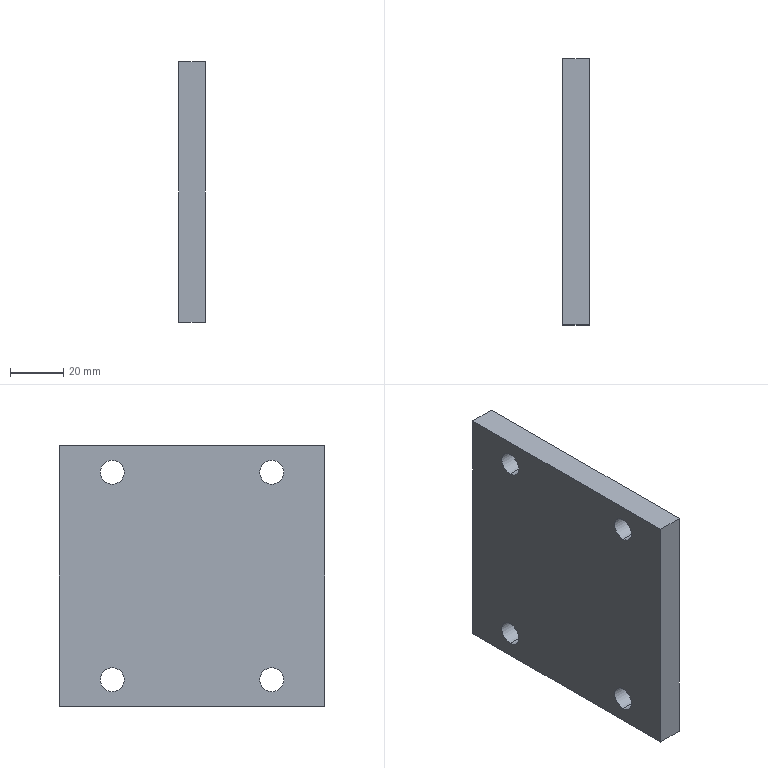Part | SolidWorks | features Extrusion 1, HoleWzd 1 | 1 solid | 14 faces | box 10 x 100 x 98 mm | volume 95455 mm3 | cylinder 8 | plane 6 | commonest cylinder face diameters 9 x8
STEP:
#1=CARTESIAN_POINT('',(0.,30.,43.5));
#2=VERTEX_POINT('',#1);
#3=CARTESIAN_POINT('',(0.,30.,34.5));
#4=VERTEX_POINT('',#3);
#5=CARTESIAN_POINT('',(0.,30.,39.));
#6=DIRECTION('',(1.,0.,0.));
#7=DIRECTION('',(0.,0.,-1.));
#8=AXIS2_PLACEMENT_3D('',#5,#6,#7);
#9=CIRCLE('',#8,4.5);
#10=EDGE_CURVE('',#2,#4,#9,.T.);
#11=ORIENTED_EDGE('',*,*,#10,.F.);
#12=CARTESIAN_POINT('',(10.,30.,43.5));
#13=VERTEX_POINT('',#12);
#14=CARTESIAN_POINT('',(10.,30.,43.5));
#15=DIRECTION('',(1.,0.,0.));
#16=VECTOR('',#15,1000.);
#17=LINE('',#14,#16);
#18=EDGE_CURVE('',#2,#13,#17,.T.);
#19=ORIENTED_EDGE('',*,*,#18,.T.);
#20=CARTESIAN_POINT('',(10.,30.,34.5));
#21=VERTEX_POINT('',#20);
#22=CARTESIAN_POINT('',(10.,30.,39.));
#23=DIRECTION('',(1.,0.,0.));
#24=DIRECTION('',(0.,0.,-1.));
#25=AXIS2_PLACEMENT_3D('',#22,#23,#24);
#26=CIRCLE('',#25,4.5);
#27=EDGE_CURVE('',#13,#21,#26,.T.);
#28=ORIENTED_EDGE('',*,*,#27,.T.);
#29=CARTESIAN_POINT('',(10.,30.,34.5));
#30=DIRECTION('',(1.,0.,0.));
#31=VECTOR('',#30,1000.);
#32=LINE('',#29,#31);
#33=EDGE_CURVE('',#4,#21,#32,.T.);
#34=ORIENTED_EDGE('',*,*,#33,.F.);
#35=EDGE_LOOP('',(#11,#19,#28,#34));
#36=FACE_OUTER_BOUND('',#35,.T.);
#37=CARTESIAN_POINT('',(10.,30.,39.));
#38=DIRECTION('',(1.,0.,0.));
#39=DIRECTION('',(0.,0.,-1.));
#40=AXIS2_PLACEMENT_3D('',#37,#38,#39);
#41=CYLINDRICAL_SURFACE('',#40,4.5);
#42=ADVANCED_FACE('',(#36),#41,.F.);
#43=CARTESIAN_POINT('',(0.,30.,-34.5));
#44=VERTEX_POINT('',#43);
#45=CARTESIAN_POINT('',(0.,30.,-43.5));
#46=VERTEX_POINT('',#45);
#47=CARTESIAN_POINT('',(0.,30.,-39.));
#48=DIRECTION('',(1.,0.,0.));
#49=DIRECTION('',(0.,0.,-1.));
#50=AXIS2_PLACEMENT_3D('',#47,#48,#49);
#51=CIRCLE('',#50,4.5);
#52=EDGE_CURVE('',#44,#46,#51,.T.);
#53=ORIENTED_EDGE('',*,*,#52,.F.);
#54=CARTESIAN_POINT('',(10.,30.,-34.5));
#55=VERTEX_POINT('',#54);
#56=CARTESIAN_POINT('',(10.,30.,-34.5));
#57=DIRECTION('',(1.,0.,0.));
#58=VECTOR('',#57,1000.);
#59=LINE('',#56,#58);
#60=EDGE_CURVE('',#44,#55,#59,.T.);
#61=ORIENTED_EDGE('',*,*,#60,.T.);
#62=CARTESIAN_POINT('',(10.,30.,-43.5));
#63=VERTEX_POINT('',#62);
#64=CARTESIAN_POINT('',(10.,30.,-39.));
#65=DIRECTION('',(1.,0.,0.));
#66=DIRECTION('',(0.,0.,-1.));
#67=AXIS2_PLACEMENT_3D('',#64,#65,#66);
#68=CIRCLE('',#67,4.5);
#69=EDGE_CURVE('',#55,#63,#68,.T.);
#70=ORIENTED_EDGE('',*,*,#69,.T.);
#71=CARTESIAN_POINT('',(10.,30.,-43.5));
#72=DIRECTION('',(1.,0.,0.));
#73=VECTOR('',#72,1000.);
#74=LINE('',#71,#73);
#75=EDGE_CURVE('',#46,#63,#74,.T.);
#76=ORIENTED_EDGE('',*,*,#75,.F.);
#77=EDGE_LOOP('',(#53,#61,#70,#76));
#78=FACE_OUTER_BOUND('',#77,.T.);
#79=CARTESIAN_POINT('',(10.,30.,-39.));
#80=DIRECTION('',(1.,0.,0.));
#81=DIRECTION('',(0.,0.,-1.));
#82=AXIS2_PLACEMENT_3D('',#79,#80,#81);
#83=CYLINDRICAL_SURFACE('',#82,4.5);
#84=ADVANCED_FACE('',(#78),#83,.F.);
#85=CARTESIAN_POINT('',(0.,-30.,43.5));
#86=VERTEX_POINT('',#85);
#87=CARTESIAN_POINT('',(0.,-30.,34.5));
#88=VERTEX_POINT('',#87);
#89=CARTESIAN_POINT('',(0.,-30.,39.));
#90=DIRECTION('',(1.,0.,0.));
#91=DIRECTION('',(0.,0.,-1.));
#92=AXIS2_PLACEMENT_3D('',#89,#90,#91);
#93=CIRCLE('',#92,4.5);
#94=EDGE_CURVE('',#86,#88,#93,.T.);
#95=ORIENTED_EDGE('',*,*,#94,.F.);
#96=CARTESIAN_POINT('',(10.,-30.,43.5));
#97=VERTEX_POINT('',#96);
#98=CARTESIAN_POINT('',(10.,-30.,43.5));
#99=DIRECTION('',(1.,0.,0.));
#100=VECTOR('',#99,1000.);
#101=LINE('',#98,#100);
#102=EDGE_CURVE('',#86,#97,#101,.T.);
#103=ORIENTED_EDGE('',*,*,#102,.T.);
#104=CARTESIAN_POINT('',(10.,-30.,34.5));
#105=VERTEX_POINT('',#104);
#106=CARTESIAN_POINT('',(10.,-30.,39.));
#107=DIRECTION('',(1.,0.,0.));
#108=DIRECTION('',(0.,0.,-1.));
#109=AXIS2_PLACEMENT_3D('',#106,#107,#108);
#110=CIRCLE('',#109,4.5);
#111=EDGE_CURVE('',#97,#105,#110,.T.);
#112=ORIENTED_EDGE('',*,*,#111,.T.);
#113=CARTESIAN_POINT('',(10.,-30.,34.5));
#114=DIRECTION('',(1.,0.,0.));
#115=VECTOR('',#114,1000.);
#116=LINE('',#113,#115);
#117=EDGE_CURVE('',#88,#105,#116,.T.);
#118=ORIENTED_EDGE('',*,*,#117,.F.);
#119=EDGE_LOOP('',(#95,#103,#112,#118));
#120=FACE_OUTER_BOUND('',#119,.T.);
#121=CARTESIAN_POINT('',(10.,-30.,39.));
#122=DIRECTION('',(1.,0.,0.));
#123=DIRECTION('',(0.,0.,-1.));
#124=AXIS2_PLACEMENT_3D('',#121,#122,#123);
#125=CYLINDRICAL_SURFACE('',#124,4.5);
#126=ADVANCED_FACE('',(#120),#125,.F.);
#127=CARTESIAN_POINT('',(0.,-30.,-34.5));
#128=VERTEX_POINT('',#127);
#129=CARTESIAN_POINT('',(0.,-30.,-43.5));
#130=VERTEX_POINT('',#129);
#131=CARTESIAN_POINT('',(0.,-30.,-39.));
#132=DIRECTION('',(1.,0.,0.));
#133=DIRECTION('',(0.,0.,-1.));
#134=AXIS2_PLACEMENT_3D('',#131,#132,#133);
#135=CIRCLE('',#134,4.5);
#136=EDGE_CURVE('',#128,#130,#135,.T.);
#137=ORIENTED_EDGE('',*,*,#136,.F.);
#138=CARTESIAN_POINT('',(10.,-30.,-34.5));
#139=VERTEX_POINT('',#138);
#140=CARTESIAN_POINT('',(10.,-30.,-34.5));
#141=DIRECTION('',(1.,0.,0.));
#142=VECTOR('',#141,1000.);
#143=LINE('',#140,#142);
#144=EDGE_CURVE('',#128,#139,#143,.T.);
#145=ORIENTED_EDGE('',*,*,#144,.T.);
#146=CARTESIAN_POINT('',(10.,-30.,-43.5));
#147=VERTEX_POINT('',#146);
#148=CARTESIAN_POINT('',(10.,-30.,-39.));
#149=DIRECTION('',(1.,0.,0.));
#150=DIRECTION('',(0.,0.,-1.));
#151=AXIS2_PLACEMENT_3D('',#148,#149,#150);
#152=CIRCLE('',#151,4.5);
#153=EDGE_CURVE('',#139,#147,#152,.T.);
#154=ORIENTED_EDGE('',*,*,#153,.T.);
#155=CARTESIAN_POINT('',(10.,-30.,-43.5));
#156=DIRECTION('',(1.,0.,0.));
#157=VECTOR('',#156,1000.);
#158=LINE('',#155,#157);
#159=EDGE_CURVE('',#130,#147,#158,.T.);
#160=ORIENTED_EDGE('',*,*,#159,.F.);
#161=EDGE_LOOP('',(#137,#145,#154,#160));
#162=FACE_OUTER_BOUND('',#161,.T.);
#163=CARTESIAN_POINT('',(10.,-30.,-39.));
#164=DIRECTION('',(1.,0.,0.));
#165=DIRECTION('',(0.,0.,-1.));
#166=AXIS2_PLACEMENT_3D('',#163,#164,#165);
#167=CYLINDRICAL_SURFACE('',#166,4.5);
#168=ADVANCED_FACE('',(#162),#167,.F.);
#169=CARTESIAN_POINT('',(0.,-50.,-49.));
#170=VERTEX_POINT('',#169);
#171=CARTESIAN_POINT('',(0.,50.,-49.));
#172=VERTEX_POINT('',#171);
#173=CARTESIAN_POINT('',(0.,50.,-49.));
#174=DIRECTION('',(0.,1.,0.));
#175=VECTOR('',#174,1000.);
#176=LINE('',#173,#175);
#177=EDGE_CURVE('',#170,#172,#176,.T.);
#178=ORIENTED_EDGE('',*,*,#177,.T.);
#179=CARTESIAN_POINT('',(10.,50.,-49.));
#180=VERTEX_POINT('',#179);
#181=CARTESIAN_POINT('',(10.,50.,-49.));
#182=DIRECTION('',(-1.,0.,0.));
#183=VECTOR('',#182,1000.);
#184=LINE('',#181,#183);
#185=EDGE_CURVE('',#180,#172,#184,.T.);
#186=ORIENTED_EDGE('',*,*,#185,.F.);
#187=CARTESIAN_POINT('',(10.,-50.,-49.));
#188=VERTEX_POINT('',#187);
#189=CARTESIAN_POINT('',(10.,50.,-49.));
#190=DIRECTION('',(0.,1.,0.));
#191=VECTOR('',#190,1000.);
#192=LINE('',#189,#191);
#193=EDGE_CURVE('',#188,#180,#192,.T.);
#194=ORIENTED_EDGE('',*,*,#193,.F.);
#195=CARTESIAN_POINT('',(10.,-50.,-49.));
#196=DIRECTION('',(-1.,0.,0.));
#197=VECTOR('',#196,1000.);
#198=LINE('',#195,#197);
#199=EDGE_CURVE('',#188,#170,#198,.T.);
#200=ORIENTED_EDGE('',*,*,#199,.T.);
#201=EDGE_LOOP('',(#178,#186,#194,#200));
#202=FACE_OUTER_BOUND('',#201,.T.);
#203=CARTESIAN_POINT('',(10.,50.,-49.));
#204=DIRECTION('',(0.,0.,1.));
#205=DIRECTION('',(0.,-1.,0.));
#206=AXIS2_PLACEMENT_3D('',#203,#204,#205);
#207=PLANE('',#206);
#208=ADVANCED_FACE('',(#202),#207,.F.);
#209=CARTESIAN_POINT('',(0.,50.,49.));
#210=VERTEX_POINT('',#209);
#211=CARTESIAN_POINT('',(0.,50.,49.));
#212=DIRECTION('',(0.,0.,1.));
#213=VECTOR('',#212,1000.);
#214=LINE('',#211,#213);
#215=EDGE_CURVE('',#172,#210,#214,.T.);
#216=ORIENTED_EDGE('',*,*,#215,.T.);
#217=CARTESIAN_POINT('',(10.,50.,49.));
#218=VERTEX_POINT('',#217);
#219=CARTESIAN_POINT('',(10.,50.,49.));
#220=DIRECTION('',(-1.,0.,0.));
#221=VECTOR('',#220,1000.);
#222=LINE('',#219,#221);
#223=EDGE_CURVE('',#218,#210,#222,.T.);
#224=ORIENTED_EDGE('',*,*,#223,.F.);
#225=CARTESIAN_POINT('',(10.,50.,49.));
#226=DIRECTION('',(0.,0.,1.));
#227=VECTOR('',#226,1000.);
#228=LINE('',#225,#227);
#229=EDGE_CURVE('',#180,#218,#228,.T.);
#230=ORIENTED_EDGE('',*,*,#229,.F.);
#231=ORIENTED_EDGE('',*,*,#185,.T.);
#232=EDGE_LOOP('',(#216,#224,#230,#231));
#233=FACE_OUTER_BOUND('',#232,.T.);
#234=CARTESIAN_POINT('',(10.,50.,49.));
#235=DIRECTION('',(0.,-1.,0.));
#236=DIRECTION('',(0.,0.,-1.));
#237=AXIS2_PLACEMENT_3D('',#234,#235,#236);
#238=PLANE('',#237);
#239=ADVANCED_FACE('',(#233),#238,.F.);
#240=CARTESIAN_POINT('',(0.,-50.,49.));
#241=VERTEX_POINT('',#240);
#242=CARTESIAN_POINT('',(0.,50.,49.));
#243=DIRECTION('',(0.,-1.,0.));
#244=VECTOR('',#243,1000.);
#245=LINE('',#242,#244);
#246=EDGE_CURVE('',#210,#241,#245,.T.);
#247=ORIENTED_EDGE('',*,*,#246,.T.);
#248=CARTESIAN_POINT('',(10.,-50.,49.));
#249=VERTEX_POINT('',#248);
#250=CARTESIAN_POINT('',(10.,-50.,49.));
#251=DIRECTION('',(-1.,0.,0.));
#252=VECTOR('',#251,1000.);
#253=LINE('',#250,#252);
#254=EDGE_CURVE('',#249,#241,#253,.T.);
#255=ORIENTED_EDGE('',*,*,#254,.F.);
#256=CARTESIAN_POINT('',(10.,50.,49.));
#257=DIRECTION('',(0.,-1.,0.));
#258=VECTOR('',#257,1000.);
#259=LINE('',#256,#258);
#260=EDGE_CURVE('',#218,#249,#259,.T.);
#261=ORIENTED_EDGE('',*,*,#260,.F.);
#262=ORIENTED_EDGE('',*,*,#223,.T.);
#263=EDGE_LOOP('',(#247,#255,#261,#262));
#264=FACE_OUTER_BOUND('',#263,.T.);
#265=CARTESIAN_POINT('',(10.,50.,49.));
#266=DIRECTION('',(0.,0.,-1.));
#267=DIRECTION('',(0.,1.,0.));
#268=AXIS2_PLACEMENT_3D('',#265,#266,#267);
#269=PLANE('',#268);
#270=ADVANCED_FACE('',(#264),#269,.F.);
#271=CARTESIAN_POINT('',(0.,-50.,49.));
#272=DIRECTION('',(0.,0.,-1.));
#273=VECTOR('',#272,1000.);
#274=LINE('',#271,#273);
#275=EDGE_CURVE('',#241,#170,#274,.T.);
#276=ORIENTED_EDGE('',*,*,#275,.T.);
#277=ORIENTED_EDGE('',*,*,#199,.F.);
#278=CARTESIAN_POINT('',(10.,-50.,49.));
#279=DIRECTION('',(0.,0.,-1.));
#280=VECTOR('',#279,1000.);
#281=LINE('',#278,#280);
#282=EDGE_CURVE('',#249,#188,#281,.T.);
#283=ORIENTED_EDGE('',*,*,#282,.F.);
#284=ORIENTED_EDGE('',*,*,#254,.T.);
#285=EDGE_LOOP('',(#276,#277,#283,#284));
#286=FACE_OUTER_BOUND('',#285,.T.);
#287=CARTESIAN_POINT('',(10.,-50.,49.));
#288=DIRECTION('',(0.,1.,0.));
#289=DIRECTION('',(0.,0.,1.));
#290=AXIS2_PLACEMENT_3D('',#287,#288,#289);
#291=PLANE('',#290);
#292=ADVANCED_FACE('',(#286),#291,.F.);
#293=CARTESIAN_POINT('',(10.,30.,39.));
#294=DIRECTION('',(1.,0.,0.));
#295=DIRECTION('',(0.,0.,-1.));
#296=AXIS2_PLACEMENT_3D('',#293,#294,#295);
#297=CIRCLE('',#296,4.5);
#298=EDGE_CURVE('',#21,#13,#297,.T.);
#299=ORIENTED_EDGE('',*,*,#298,.F.);
#300=ORIENTED_EDGE('',*,*,#27,.F.);
#301=EDGE_LOOP('',(#299,#300));
#302=FACE_BOUND('',#301,.T.);
#303=CARTESIAN_POINT('',(10.,30.,-39.));
#304=DIRECTION('',(1.,0.,0.));
#305=DIRECTION('',(0.,0.,-1.));
#306=AXIS2_PLACEMENT_3D('',#303,#304,#305);
#307=CIRCLE('',#306,4.5);
#308=EDGE_CURVE('',#63,#55,#307,.T.);
#309=ORIENTED_EDGE('',*,*,#308,.F.);
#310=ORIENTED_EDGE('',*,*,#69,.F.);
#311=EDGE_LOOP('',(#309,#310));
#312=FACE_BOUND('',#311,.T.);
#313=CARTESIAN_POINT('',(10.,-30.,39.));
#314=DIRECTION('',(1.,0.,0.));
#315=DIRECTION('',(0.,0.,-1.));
#316=AXIS2_PLACEMENT_3D('',#313,#314,#315);
#317=CIRCLE('',#316,4.5);
#318=EDGE_CURVE('',#105,#97,#317,.T.);
#319=ORIENTED_EDGE('',*,*,#318,.F.);
#320=ORIENTED_EDGE('',*,*,#111,.F.);
#321=EDGE_LOOP('',(#319,#320));
#322=FACE_BOUND('',#321,.T.);
#323=CARTESIAN_POINT('',(10.,-30.,-39.));
#324=DIRECTION('',(1.,0.,0.));
#325=DIRECTION('',(0.,0.,-1.));
#326=AXIS2_PLACEMENT_3D('',#323,#324,#325);
#327=CIRCLE('',#326,4.5);
#328=EDGE_CURVE('',#147,#139,#327,.T.);
#329=ORIENTED_EDGE('',*,*,#328,.F.);
#330=ORIENTED_EDGE('',*,*,#153,.F.);
#331=EDGE_LOOP('',(#329,#330));
#332=FACE_BOUND('',#331,.T.);
#333=ORIENTED_EDGE('',*,*,#193,.T.);
#334=ORIENTED_EDGE('',*,*,#229,.T.);
#335=ORIENTED_EDGE('',*,*,#260,.T.);
#336=ORIENTED_EDGE('',*,*,#282,.T.);
#337=EDGE_LOOP('',(#333,#334,#335,#336));
#338=FACE_OUTER_BOUND('',#337,.T.);
#339=CARTESIAN_POINT('',(10.,0.,0.));
#340=DIRECTION('',(1.,0.,0.));
#341=DIRECTION('',(0.,0.,-1.));
#342=AXIS2_PLACEMENT_3D('',#339,#340,#341);
#343=PLANE('',#342);
#344=ADVANCED_FACE('',(#302,#312,#322,#332,#338),#343,.T.);
#345=CARTESIAN_POINT('',(0.,30.,39.));
#346=DIRECTION('',(1.,0.,0.));
#347=DIRECTION('',(0.,0.,-1.));
#348=AXIS2_PLACEMENT_3D('',#345,#346,#347);
#349=CIRCLE('',#348,4.5);
#350=EDGE_CURVE('',#4,#2,#349,.T.);
#351=ORIENTED_EDGE('',*,*,#350,.T.);
#352=ORIENTED_EDGE('',*,*,#10,.T.);
#353=EDGE_LOOP('',(#351,#352));
#354=FACE_BOUND('',#353,.T.);
#355=CARTESIAN_POINT('',(0.,30.,-39.));
#356=DIRECTION('',(1.,0.,0.));
#357=DIRECTION('',(0.,0.,-1.));
#358=AXIS2_PLACEMENT_3D('',#355,#356,#357);
#359=CIRCLE('',#358,4.5);
#360=EDGE_CURVE('',#46,#44,#359,.T.);
#361=ORIENTED_EDGE('',*,*,#360,.T.);
#362=ORIENTED_EDGE('',*,*,#52,.T.);
#363=EDGE_LOOP('',(#361,#362));
#364=FACE_BOUND('',#363,.T.);
#365=CARTESIAN_POINT('',(0.,-30.,39.));
#366=DIRECTION('',(1.,0.,0.));
#367=DIRECTION('',(0.,0.,-1.));
#368=AXIS2_PLACEMENT_3D('',#365,#366,#367);
#369=CIRCLE('',#368,4.5);
#370=EDGE_CURVE('',#88,#86,#369,.T.);
#371=ORIENTED_EDGE('',*,*,#370,.T.);
#372=ORIENTED_EDGE('',*,*,#94,.T.);
#373=EDGE_LOOP('',(#371,#372));
#374=FACE_BOUND('',#373,.T.);
#375=CARTESIAN_POINT('',(0.,-30.,-39.));
#376=DIRECTION('',(1.,0.,0.));
#377=DIRECTION('',(0.,0.,-1.));
#378=AXIS2_PLACEMENT_3D('',#375,#376,#377);
#379=CIRCLE('',#378,4.5);
#380=EDGE_CURVE('',#130,#128,#379,.T.);
#381=ORIENTED_EDGE('',*,*,#380,.T.);
#382=ORIENTED_EDGE('',*,*,#136,.T.);
#383=EDGE_LOOP('',(#381,#382));
#384=FACE_BOUND('',#383,.T.);
#385=ORIENTED_EDGE('',*,*,#177,.F.);
#386=ORIENTED_EDGE('',*,*,#275,.F.);
#387=ORIENTED_EDGE('',*,*,#246,.F.);
#388=ORIENTED_EDGE('',*,*,#215,.F.);
#389=EDGE_LOOP('',(#385,#386,#387,#388));
#390=FACE_OUTER_BOUND('',#389,.T.);
#391=CARTESIAN_POINT('',(0.,0.,0.));
#392=DIRECTION('',(1.,0.,0.));
#393=DIRECTION('',(0.,0.,-1.));
#394=AXIS2_PLACEMENT_3D('',#391,#392,#393);
#395=PLANE('',#394);
#396=ADVANCED_FACE('',(#354,#364,#374,#384,#390),#395,.F.);
#397=ORIENTED_EDGE('',*,*,#144,.F.);
#398=ORIENTED_EDGE('',*,*,#380,.F.);
#399=ORIENTED_EDGE('',*,*,#159,.T.);
#400=ORIENTED_EDGE('',*,*,#328,.T.);
#401=EDGE_LOOP('',(#397,#398,#399,#400));
#402=FACE_OUTER_BOUND('',#401,.T.);
#403=CARTESIAN_POINT('',(10.,-30.,-39.));
#404=DIRECTION('',(1.,0.,0.));
#405=DIRECTION('',(0.,0.,-1.));
#406=AXIS2_PLACEMENT_3D('',#403,#404,#405);
#407=CYLINDRICAL_SURFACE('',#406,4.5);
#408=ADVANCED_FACE('',(#402),#407,.F.);
#409=ORIENTED_EDGE('',*,*,#102,.F.);
#410=ORIENTED_EDGE('',*,*,#370,.F.);
#411=ORIENTED_EDGE('',*,*,#117,.T.);
#412=ORIENTED_EDGE('',*,*,#318,.T.);
#413=EDGE_LOOP('',(#409,#410,#411,#412));
#414=FACE_OUTER_BOUND('',#413,.T.);
#415=CARTESIAN_POINT('',(10.,-30.,39.));
#416=DIRECTION('',(1.,0.,0.));
#417=DIRECTION('',(0.,0.,-1.));
#418=AXIS2_PLACEMENT_3D('',#415,#416,#417);
#419=CYLINDRICAL_SURFACE('',#418,4.5);
#420=ADVANCED_FACE('',(#414),#419,.F.);
#421=ORIENTED_EDGE('',*,*,#60,.F.);
#422=ORIENTED_EDGE('',*,*,#360,.F.);
#423=ORIENTED_EDGE('',*,*,#75,.T.);
#424=ORIENTED_EDGE('',*,*,#308,.T.);
#425=EDGE_LOOP('',(#421,#422,#423,#424));
#426=FACE_OUTER_BOUND('',#425,.T.);
#427=CARTESIAN_POINT('',(10.,30.,-39.));
#428=DIRECTION('',(1.,0.,0.));
#429=DIRECTION('',(0.,0.,-1.));
#430=AXIS2_PLACEMENT_3D('',#427,#428,#429);
#431=CYLINDRICAL_SURFACE('',#430,4.5);
#432=ADVANCED_FACE('',(#426),#431,.F.);
#433=ORIENTED_EDGE('',*,*,#18,.F.);
#434=ORIENTED_EDGE('',*,*,#350,.F.);
#435=ORIENTED_EDGE('',*,*,#33,.T.);
#436=ORIENTED_EDGE('',*,*,#298,.T.);
#437=EDGE_LOOP('',(#433,#434,#435,#436));
#438=FACE_OUTER_BOUND('',#437,.T.);
#439=CARTESIAN_POINT('',(10.,30.,39.));
#440=DIRECTION('',(1.,0.,0.));
#441=DIRECTION('',(0.,0.,-1.));
#442=AXIS2_PLACEMENT_3D('',#439,#440,#441);
#443=CYLINDRICAL_SURFACE('',#442,4.5);
#444=ADVANCED_FACE('',(#438),#443,.F.);
#445=CLOSED_SHELL('',(#42,#84,#126,#168,#208,#239,#270,#292,#344,#396,#408,#420,#432,#444));
#446=MANIFOLD_SOLID_BREP('',#445);
#447=CARTESIAN_POINT('',(0.,0.,0.));
#448=DIRECTION('',(0.,0.,1.));
#449=DIRECTION('',(1.,0.,0.));
#450=AXIS2_PLACEMENT_3D('',#447,#448,#449);
#451=(LENGTH_UNIT()NAMED_UNIT(*)SI_UNIT(.MILLI.,.METRE.));
#452=UNCERTAINTY_MEASURE_WITH_UNIT(LENGTH_MEASURE(0.00001),#451,'','');
#453=(NAMED_UNIT(*)PLANE_ANGLE_UNIT()SI_UNIT($,.RADIAN.));
#454=(NAMED_UNIT(*)SI_UNIT($,.STERADIAN.)SOLID_ANGLE_UNIT());
#455=(GEOMETRIC_REPRESENTATION_CONTEXT(3)GLOBAL_UNCERTAINTY_ASSIGNED_CONTEXT((#452))GLOBAL_UNIT_ASSIGNED_CONTEXT((#451,#453,#454))REPRESENTATION_CONTEXT('',''));
#456=ADVANCED_BREP_SHAPE_REPRESENTATION('',(#446,#450),#455);